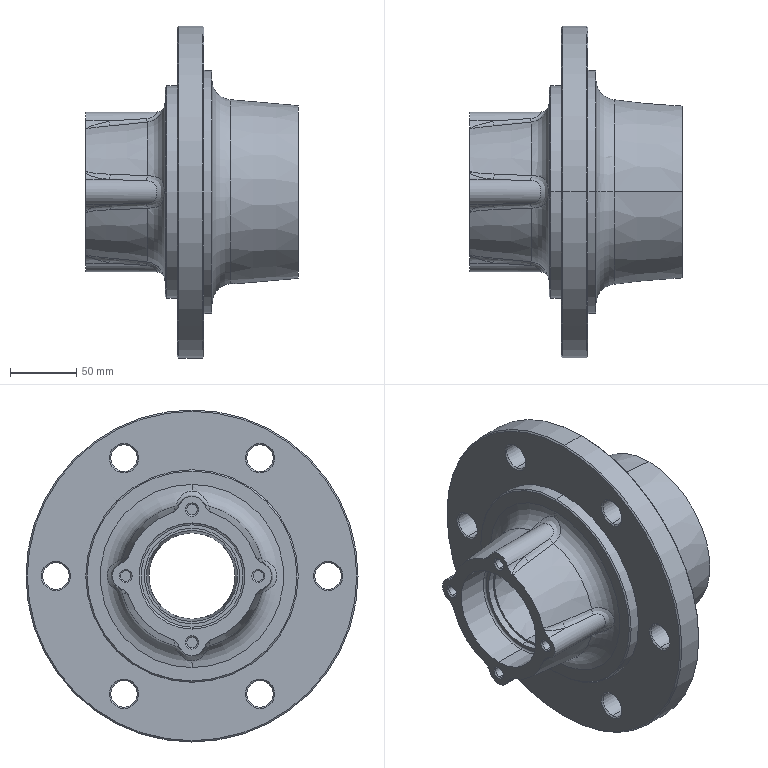Part | STEP file | AXIS_HOUSING1V11 | 1 solid | 157 faces | box 160 x 250 x 250 mm | volume 1786863 mm3 | cylinder 53 | cone 50 | spline 28 | plane 16 | torus 10 | commonest cylinder face diameters 20 x25 8 x8 10 x2 16 x2 65 x2 72 x2